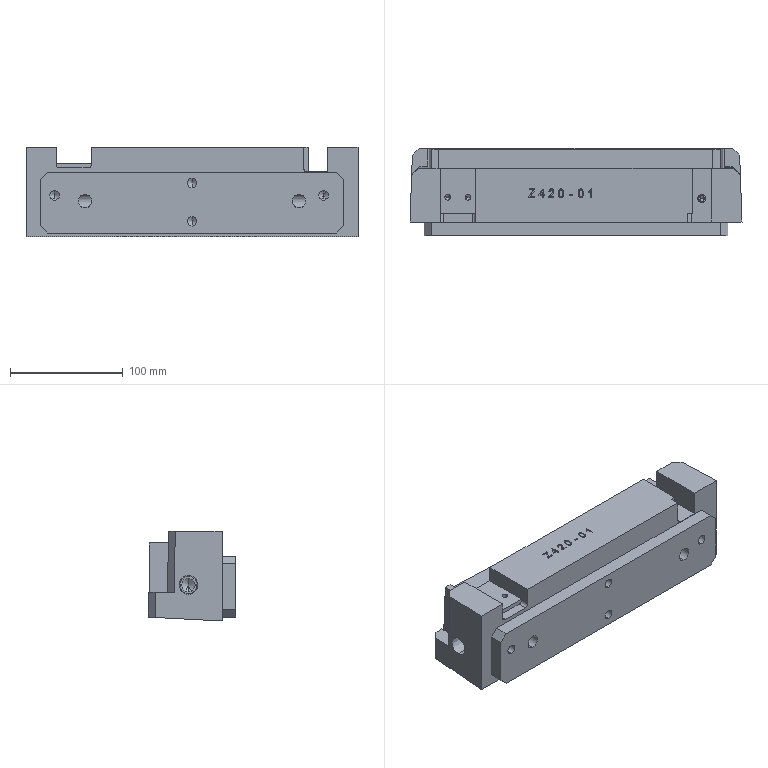Part | Creo | 1 solid | 2144 faces | box 294.997 x 77.574 x 79.966 mm | volume 1444919 mm3 | plane 1539 | other 537 | cylinder 48 | cone 20 | commonest cylinder face diameters 10.118 x10 8.5 x8 12 x8 5.1 x6 2.009 x4 21.562 x4